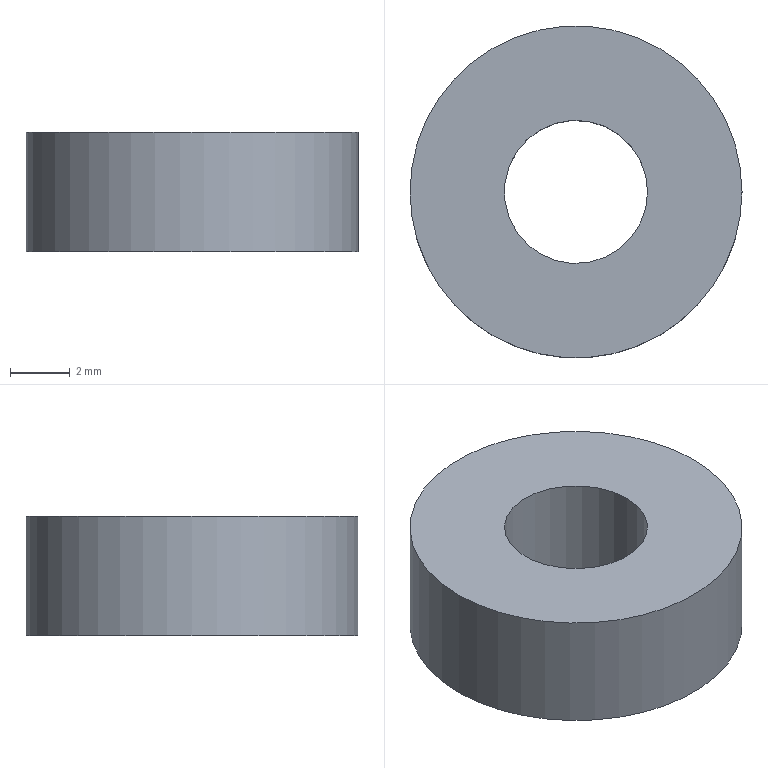Part | NX | features solid 2 | 1 solid | 4 faces | box 11.13 x 11.13 x 4 mm | volume 316.788 mm3 | cylinder 2 | plane 2 | commonest cylinder face diameters 4.8 x1 11.13 x1
STEP:
#1=CARTESIAN_POINT('',(5.565,0.,4.));
#2=VERTEX_POINT('',#1);
#3=CARTESIAN_POINT('',(0.,0.,4.));
#4=DIRECTION('',(0.,0.,1.));
#5=DIRECTION('',(1.,0.,0.));
#6=AXIS2_PLACEMENT_3D('',#3,#4,#5);
#7=CIRCLE('',#6,5.565);
#8=EDGE_CURVE('',#2,#2,#7,.T.);
#9=ORIENTED_EDGE('',*,*,#8,.F.);
#10=EDGE_LOOP('',(#9));
#11=FACE_BOUND('',#10,.T.);
#12=CARTESIAN_POINT('',(5.565,0.,0.));
#13=VERTEX_POINT('',#12);
#14=CARTESIAN_POINT('',(0.,0.,0.));
#15=DIRECTION('',(0.,0.,1.));
#16=DIRECTION('',(1.,0.,0.));
#17=AXIS2_PLACEMENT_3D('',#14,#15,#16);
#18=CIRCLE('',#17,5.565);
#19=EDGE_CURVE('',#13,#13,#18,.T.);
#20=ORIENTED_EDGE('',*,*,#19,.T.);
#21=EDGE_LOOP('',(#20));
#22=FACE_BOUND('',#21,.T.);
#23=CARTESIAN_POINT('',(0.,0.,4.));
#24=DIRECTION('',(0.,0.,-1.));
#25=DIRECTION('',(-1.,0.,0.));
#26=AXIS2_PLACEMENT_3D('',#23,#24,#25);
#27=CYLINDRICAL_SURFACE('',#26,5.565);
#28=ADVANCED_FACE('',(#11,#22),#27,.T.);
#29=CARTESIAN_POINT('',(2.4,0.,4.));
#30=VERTEX_POINT('',#29);
#31=CARTESIAN_POINT('',(0.,0.,4.));
#32=DIRECTION('',(0.,0.,1.));
#33=DIRECTION('',(1.,0.,0.));
#34=AXIS2_PLACEMENT_3D('',#31,#32,#33);
#35=CIRCLE('',#34,2.4);
#36=EDGE_CURVE('',#30,#30,#35,.T.);
#37=ORIENTED_EDGE('',*,*,#36,.T.);
#38=EDGE_LOOP('',(#37));
#39=FACE_BOUND('',#38,.T.);
#40=CARTESIAN_POINT('',(2.4,0.,0.));
#41=VERTEX_POINT('',#40);
#42=CARTESIAN_POINT('',(0.,0.,0.));
#43=DIRECTION('',(0.,0.,1.));
#44=DIRECTION('',(1.,0.,0.));
#45=AXIS2_PLACEMENT_3D('',#42,#43,#44);
#46=CIRCLE('',#45,2.4);
#47=EDGE_CURVE('',#41,#41,#46,.T.);
#48=ORIENTED_EDGE('',*,*,#47,.F.);
#49=EDGE_LOOP('',(#48));
#50=FACE_BOUND('',#49,.T.);
#51=CARTESIAN_POINT('',(0.,0.,4.));
#52=DIRECTION('',(0.,0.,-1.));
#53=DIRECTION('',(-1.,0.,0.));
#54=AXIS2_PLACEMENT_3D('',#51,#52,#53);
#55=CYLINDRICAL_SURFACE('',#54,2.4);
#56=ADVANCED_FACE('',(#39,#50),#55,.F.);
#57=ORIENTED_EDGE('',*,*,#8,.T.);
#58=EDGE_LOOP('',(#57));
#59=FACE_BOUND('',#58,.T.);
#60=ORIENTED_EDGE('',*,*,#36,.F.);
#61=EDGE_LOOP('',(#60));
#62=FACE_BOUND('',#61,.T.);
#63=CARTESIAN_POINT('',(0.,0.,4.));
#64=DIRECTION('',(0.,0.,1.));
#65=DIRECTION('',(1.,0.,0.));
#66=AXIS2_PLACEMENT_3D('',#63,#64,#65);
#67=PLANE('',#66);
#68=ADVANCED_FACE('',(#59,#62),#67,.T.);
#69=ORIENTED_EDGE('',*,*,#19,.F.);
#70=EDGE_LOOP('',(#69));
#71=FACE_BOUND('',#70,.T.);
#72=ORIENTED_EDGE('',*,*,#47,.T.);
#73=EDGE_LOOP('',(#72));
#74=FACE_BOUND('',#73,.T.);
#75=CARTESIAN_POINT('',(0.,0.,0.));
#76=DIRECTION('',(0.,0.,1.));
#77=DIRECTION('',(1.,0.,0.));
#78=AXIS2_PLACEMENT_3D('',#75,#76,#77);
#79=PLANE('',#78);
#80=ADVANCED_FACE('',(#71,#74),#79,.F.);
#81=CLOSED_SHELL('',(#28,#56,#68,#80));
#82=MANIFOLD_SOLID_BREP('',#81);
#83=(LENGTH_UNIT()NAMED_UNIT(*)SI_UNIT(.MILLI.,.METRE.));
#84=UNCERTAINTY_MEASURE_WITH_UNIT(LENGTH_MEASURE(0.00001),#83,'','');
#85=(NAMED_UNIT(*)PLANE_ANGLE_UNIT()SI_UNIT($,.RADIAN.));
#86=(NAMED_UNIT(*)SI_UNIT($,.STERADIAN.)SOLID_ANGLE_UNIT());
#87=(GEOMETRIC_REPRESENTATION_CONTEXT(3)GLOBAL_UNCERTAINTY_ASSIGNED_CONTEXT((#84))GLOBAL_UNIT_ASSIGNED_CONTEXT((#83,#85,#86))REPRESENTATION_CONTEXT('',''));
#88=ADVANCED_BREP_SHAPE_REPRESENTATION('',(#82),#87);